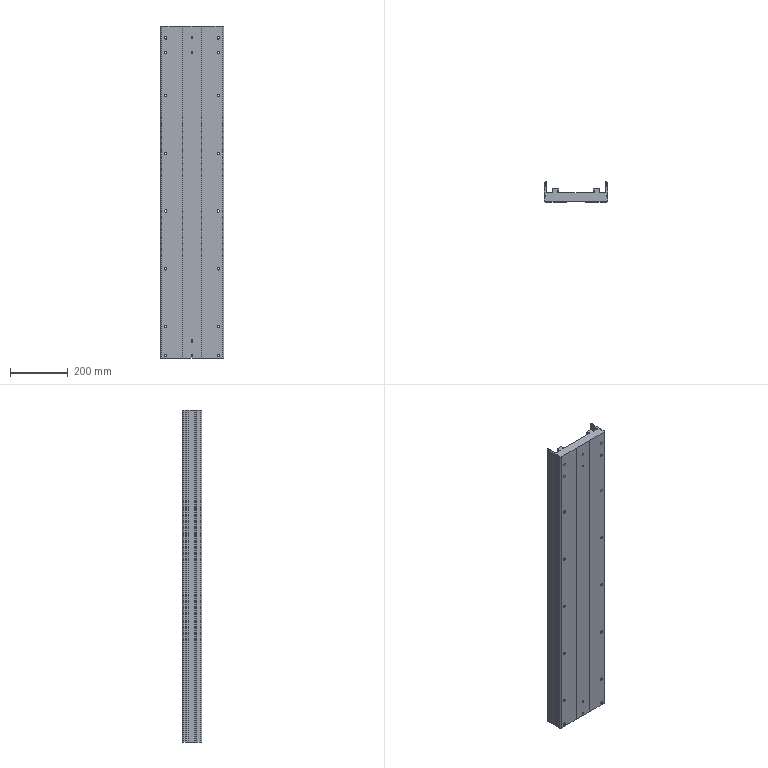Part | SolidWorks | features HoleWzd 3, ICE 3, Extrusion 1, Fillet 1, LPattern 1 | 1 solid | 222 faces | box 220 x 67.5 x 1150 mm | volume 8709767 mm3 | plane 116 | cylinder 106 | commonest cylinder face diameters 8.6 x32 15 x32 0.4 x12 6 x10 4.2 x9 10 x4